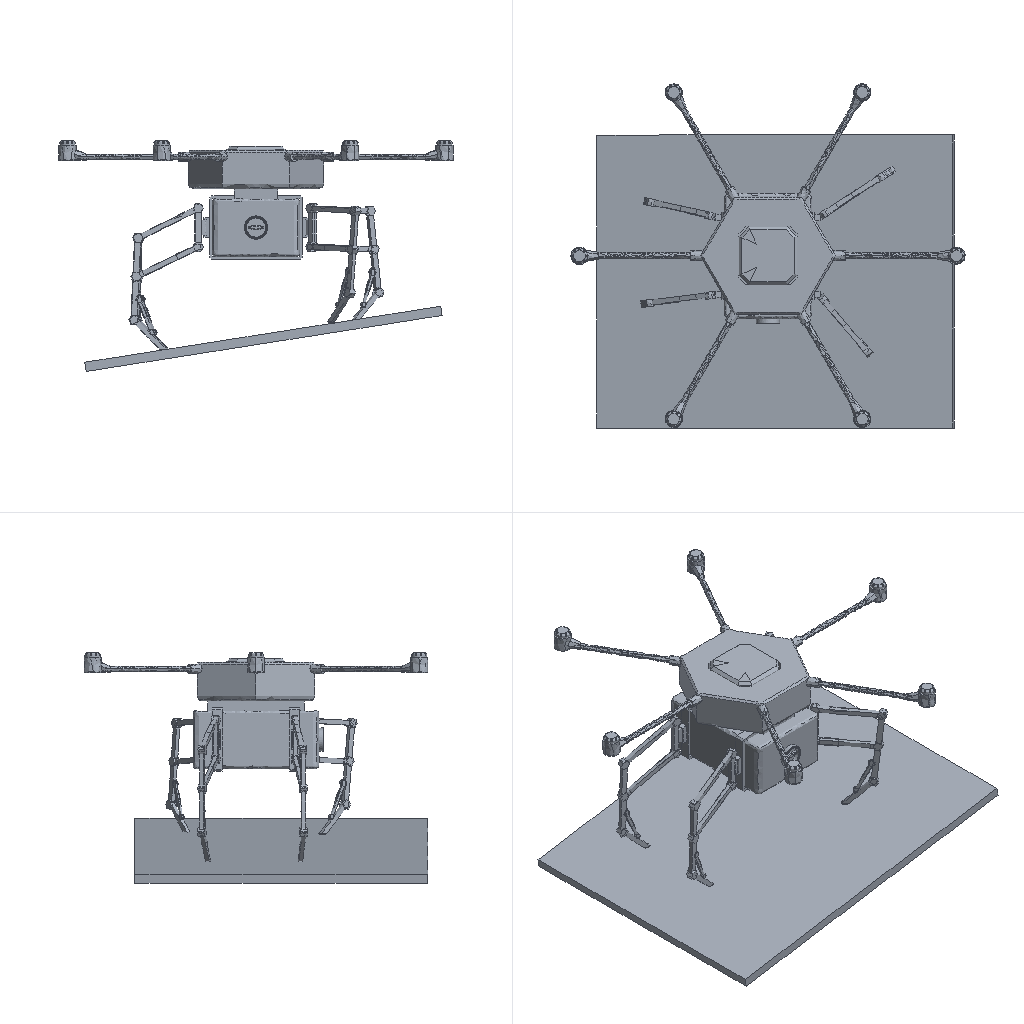Simulation study | ansys workbench
Ansys APDL input file, long lists of numbers shortened:
/batch
/config,noeldb,1     ! force off writing results to database
*get,_wallstrt,active,,time,wall
! ANSYS input file written by Workbench version 2022 R1
! File used for geometry attach:
/title,wbnew--__ (G5)
! ****** Begin Custom Load Command Snippet ******
/COM, ACT Extensions:
/COM,     LSDYNA, 2021.1
/COM,
! ****** End   Custom Load Command Snippet ******
*DIM,_wb_ProjectScratch_dir,string,248
_wb_ProjectScratch_dir(1) = ''
*DIM,_wb_SolverFiles_dir,string,248
_wb_SolverFiles_dir(1) = ''
*DIM,_wb_userfiles_dir,string,248
_wb_userfiles_dir(1) = ''
/com,--- Data in consistent NMM units. See Solving Units in the help system for more information.
/units,MPA
/nopr
/wb,file,start              !  signify a WB generated input file
/prep7
! Turn off shape checking because checks already performed inside WB mesher.
! See help system for more information.
SHPP,OFF,,NOWARN
/nolist
etcon,set             ! allow ANSYS to choose best KEYOP's for 180x elements, resets any applicable keyopt to MAPDL defaults
/com,*********** Nodes for the whole assembly ***********
nblock,3,,112522
(1i9,3e20.9e3)
        1    -5.508865346E+03    -1.475800000E+03    -1.735902488E+03
! (102292 more lines like these left out)
-1
/wb,elem,start            !  set before creation of elements
/com,*********** Elements for Body 1 "xuanyi|dianjizhijia|Chamfer.1" ***********
et,1,187
eblock,19,solid,,480
(19i9)
        1        1        1        1        0        0        0        0       10        0     5151    10218    10222    10326    10253    10413    10440    10416    10414
! (959 more lines like these left out)
-1
/com,*********** Elements for Body 2 "xuanyi|jibi|Pad.1" ***********
et,2,187
eblock,19,solid,,1308
(19i9)
        2        2        2        2        0        0        0        0       10        0    42302    78291    78292    78359    78451    79365    79376    79367    79371
! (2615 more lines like these left out)
-1
/com,*********** Elements for Body 3 "xuanyi|xuanyidianji|CircPattern.1" ***********
et,3,187
eblock,19,solid,,3493
(19i9)
        3        3        3        3        0        0        0        0       10        0     9787    19116    19133    19215    19181    23808    23876    23812    23809
! (6985 more lines like these left out)
-1
/com,*********** Elements for Body 4 "xuanyi|dianjizhijia|Chamfer.1[2]" ***********
et,4,187
eblock,19,solid,,480
(19i9)
        4        4        4        4        0        0        0        0       10        0     4671     9210     9214     9318     9245     9405     9432     9408     9406
! (959 more lines like these left out)
-1
/com,*********** Elements for Body 5 "xuanyi|jibi|Pad.1[2]" ***********
et,5,187
eblock,19,solid,,1308
(19i9)
        5        5        5        5        0        0        0        0       10        0    38378    70386    70387    70454    70546    71460    71471    71462    71466
! (2615 more lines like these left out)
-1
! (50 more sections like these left out)
/wb,elem,end               !  done creating elements
/com,*********** Send User Defined Coordinate System(s) ***********
csys,0
toffst,273.15,  ! Temperature offset from absolute zero
/com,*********** Set Reference Temperature ***********
tref,22.
/wb,mat,start              !  starting to send materials
/com,*********** Send Materials ***********
Temperature = 'TEMP' ! Temperature
MP,DENS,1,7.85e-09,	! tonne mm^-3
MP,ALPX,1,1.2e-05,	! C^-1
MP,C,1,434000000,	! mm^2 s^-2 C^-1
MP,KXX,1,60.5,	! tonne mm s^-3 C^-1
MP,RSVX,1,0.00017,	! ohm mm
MP,EX,1,200000,	! tonne s^-2 mm^-1
MP,NUXY,1,0.3,
MP,MURX,1,10000,
Temperature = 'TEMP' ! Temperature
MP,DENS,2,7.85e-09,	! tonne mm^-3
MP,ALPX,2,1.2e-05,	! C^-1
MP,C,2,434000000,	! mm^2 s^-2 C^-1
MP,KXX,2,60.5,	! tonne mm s^-3 C^-1
MP,RSVX,2,0.00017,	! ohm mm
MP,EX,2,200000,	! tonne s^-2 mm^-1
MP,NUXY,2,0.3,
MP,MURX,2,10000,
Temperature = 'TEMP' ! Temperature
MP,DENS,3,7.85e-09,	! tonne mm^-3
MP,ALPX,3,1.2e-05,	! C^-1
MP,C,3,434000000,	! mm^2 s^-2 C^-1
MP,KXX,3,60.5,	! tonne mm s^-3 C^-1
MP,RSVX,3,0.00017,	! ohm mm
MP,EX,3,200000,	! tonne s^-2 mm^-1
MP,NUXY,3,0.3,
MP,MURX,3,10000,
Temperature = 'TEMP' ! Temperature
MP,DENS,4,7.85e-09,	! tonne mm^-3
MP,ALPX,4,1.2e-05,	! C^-1
MP,C,4,434000000,	! mm^2 s^-2 C^-1
MP,KXX,4,60.5,	! tonne mm s^-3 C^-1
MP,RSVX,4,0.00017,	! ohm mm
MP,EX,4,200000,	! tonne s^-2 mm^-1
MP,NUXY,4,0.3,
MP,MURX,4,10000,
Temperature = 'TEMP' ! Temperature
MP,DENS,5,7.85e-09,	! tonne mm^-3
MP,ALPX,5,1.2e-05,	! C^-1
MP,C,5,434000000,	! mm^2 s^-2 C^-1
MP,KXX,5,60.5,	! tonne mm s^-3 C^-1
MP,RSVX,5,0.00017,	! ohm mm
MP,EX,5,200000,	! tonne s^-2 mm^-1
MP,NUXY,5,0.3,
MP,MURX,5,10000,
Temperature = 'TEMP' ! Temperature
MP,DENS,6,7.85e-09,	! tonne mm^-3
MP,ALPX,6,1.2e-05,	! C^-1
MP,C,6,434000000,	! mm^2 s^-2 C^-1
MP,KXX,6,60.5,	! tonne mm s^-3 C^-1
MP,RSVX,6,0.00017,	! ohm mm
MP,EX,6,200000,	! tonne s^-2 mm^-1
MP,NUXY,6,0.3,
MP,MURX,6,10000,
Temperature = 'TEMP' ! Temperature
MP,DENS,7,7.85e-09,	! tonne mm^-3
MP,ALPX,7,1.2e-05,	! C^-1
MP,C,7,434000000,	! mm^2 s^-2 C^-1
MP,KXX,7,60.5,	! tonne mm s^-3 C^-1
MP,RSVX,7,0.00017,	! ohm mm
MP,EX,7,200000,	! tonne s^-2 mm^-1
MP,NUXY,7,0.3,
MP,MURX,7,10000,
Temperature = 'TEMP' ! Temperature
MP,DENS,8,7.85e-09,	! tonne mm^-3
MP,ALPX,8,1.2e-05,	! C^-1
MP,C,8,434000000,	! mm^2 s^-2 C^-1
MP,KXX,8,60.5,	! tonne mm s^-3 C^-1
MP,RSVX,8,0.00017,	! ohm mm
MP,EX,8,200000,	! tonne s^-2 mm^-1
MP,NUXY,8,0.3,
MP,MURX,8,10000,
Temperature = 'TEMP' ! Temperature
MP,DENS,9,7.85e-09,	! tonne mm^-3
MP,ALPX,9,1.2e-05,	! C^-1
MP,C,9,434000000,	! mm^2 s^-2 C^-1
MP,KXX,9,60.5,	! tonne mm s^-3 C^-1
MP,RSVX,9,0.00017,	! ohm mm
MP,EX,9,200000,	! tonne s^-2 mm^-1
! (416 more lines like these left out)
/wb,mat,end                !  done sending materials
!************************* Model Summary ********************
!xuanyi|dianjizhijia|Chamfer.1,	结构钢,	matid,	1
!xuanyi|jibi|Pad.1,	结构钢,	matid,	2
!xuanyi|xuanyidianji|CircPattern.1,	结构钢,	matid,	3
! (54 more lines like these left out)
*get,_xmin,node,,mnloc,x
*get,_ymin,node,,mnloc,y
*get,_zmin,node,,mnloc,z
*get,_xmax,node,,mxloc,x
*get,_ymax,node,,mxloc,y
*get,_zmax,node,,mxloc,z
_ASMDIAG=(_xmax-_xmin)*(_xmax-_xmin)+(_ymax-_ymin)*(_ymax-_ymin)+(_zmax-_zmin)*(_zmax-_zmin)
_ASMDIAG=SQRT(_ASMDIAG)
/wb,contact,start          !  starting to send contact
/com,*********** Create Contact "接触区域" ***********
/com,            Real Constant Set For Above Contact Is 57 & 56
*set,tid,57
*set,cid,56
r,tid
r,cid
et,tid,170
et,cid,174
eblock,10,,,60
(15i9)
    81076       57       57       57        0    10266    10359    10268    10268    10777    10797    10268    10771
! (59 more lines like these left out)
-1
eblock,10,,,60
(15i9)
    81136       56       56       56        0    10266    10359    10268    10268    10777    10797    10268    10771
! (59 more lines like these left out)
-1
eblock,10,,,74
(15i9)
    81196       56       57       56        0    78221    78228    78223    78223    78711    78720    78223    78709
! (73 more lines like these left out)
-1
eblock,10,,,74
(15i9)
    81270       57       56       57        0    78221    78228    78223    78223    78711    78720    78223    78709
! (73 more lines like these left out)
-1
keyo,cid,8,2               ! auto create asymmetric contact (from Program Controlled setting)
keyo,cid,10,0              ! adjust contact stiffness each NR iteration (from Program Controlled setting)
keyo,cid,12,5              ! bonded always
keyo,cid,18,1              ! small sliding turned on by application
keyo,cid,2,0               ! augmented Lagrange (from Program Controlled setting)
keyo,cid,4,0               ! on Gauss point (from Program Controlled setting)
keyo,cid,9,1               ! ignore initial gaps/penetration
keyo,cid,7,0               ! No Prediction
rmod,tid,3,10.      ! FKN
rmod,tid,5,0.       ! ICONT
rmod,tid,6,0.       ! PINB
rmod,tid,10,0.      ! CNOF
rmod,tid,12,0.      ! FKT
rmod,tid,36,230     ! WB DSID
rmod,cid,3,10.      ! FKN
rmod,cid,5,0.       ! ICONT
rmod,cid,6,0.       ! PINB
rmod,cid,10,0.      ! CNOF
rmod,cid,12,0.      ! FKT
rmod,cid,36,230     ! WB DSID
/com,*********** Create Contact "接触区域 2" ***********
/com,            Real Constant Set For Above Contact Is 59 & 58
*set,tid,59
*set,cid,58
r,tid
r,cid
et,tid,170
et,cid,174
eblock,10,,,78
(15i9)
    81344       59       59       59        0    10248    10250    10360    10360    10635    10655    10360    10640
! (77 more lines like these left out)
-1
eblock,10,,,78
(15i9)
    81422       58       58       58        0    10248    10250    10360    10360    10635    10655    10360    10640
! (77 more lines like these left out)
-1
eblock,10,,,254
(15i9)
    81500       58       59       58        0    18597    18807    18604    18604    20815    20867    18604    20811
! (253 more lines like these left out)
-1
eblock,10,,,254
(15i9)
    81754       59       58       59        0    18597    18807    18604    18604    20815    20867    18604    20811
! (253 more lines like these left out)
-1
keyo,cid,8,2               ! auto create asymmetric contact (from Program Controlled setting)
keyo,cid,10,0              ! adjust contact stiffness each NR iteration (from Program Controlled setting)
keyo,cid,12,5              ! bonded always
keyo,cid,18,1              ! small sliding turned on by application
keyo,cid,2,0               ! augmented Lagrange (from Program Controlled setting)
keyo,cid,4,0               ! on Gauss point (from Program Controlled setting)
keyo,cid,9,1               ! ignore initial gaps/penetration
keyo,cid,7,0               ! No Prediction
rmod,tid,3,10.      ! FKN
rmod,tid,5,0.       ! ICONT
rmod,tid,6,0.       ! PINB
rmod,tid,10,0.      ! CNOF
rmod,tid,12,0.      ! FKT
rmod,tid,36,233     ! WB DSID
rmod,cid,3,10.      ! FKN
rmod,cid,5,0.       ! ICONT
rmod,cid,6,0.       ! PINB
rmod,cid,10,0.      ! CNOF
rmod,cid,12,0.      ! FKT
rmod,cid,36,233     ! WB DSID
/com,*********** Create Contact "接触区域 3" ***********
/com,            Real Constant Set For Above Contact Is 61 & 60
*set,tid,61
*set,cid,60
r,tid
r,cid
et,tid,170
et,cid,174
eblock,10,,,85
(15i9)
    82008       61       61       61        0    78213    78220    78218    78218    78666    78695    78218    78665
! (84 more lines like these left out)
-1
eblock,10,,,85
(15i9)
    82093       60       60       60        0    78213    78220    78218    78218    78666    78695    78218    78665
! (84 more lines like these left out)
-1
eblock,10,,,60
(15i9)
    82178       60       61       60        0    39970    40746    39973    39973    44807    44832    39973    44805
! (59 more lines like these left out)
-1
eblock,10,,,60
(15i9)
    82238       61       60       61        0    39970    40746    39973    39973    44807    44832    39973    44805
! (59 more lines like these left out)
-1
keyo,cid,8,2               ! auto create asymmetric contact (from Program Controlled setting)
keyo,cid,10,0              ! adjust contact stiffness each NR iteration (from Program Controlled setting)
keyo,cid,12,5              ! bonded always
keyo,cid,18,1              ! small sliding turned on by application
keyo,cid,2,0               ! augmented Lagrange (from Program Controlled setting)
keyo,cid,4,0               ! on Gauss point (from Program Controlled setting)
keyo,cid,9,1               ! ignore initial gaps/penetration
keyo,cid,7,0               ! No Prediction
rmod,tid,3,10.      ! FKN
rmod,tid,5,0.       ! ICONT
rmod,tid,6,0.       ! PINB
rmod,tid,10,0.      ! CNOF
rmod,tid,12,0.      ! FKT
rmod,tid,36,236     ! WB DSID
rmod,cid,3,10.      ! FKN
rmod,cid,5,0.       ! ICONT
rmod,cid,6,0.       ! PINB
rmod,cid,10,0.      ! CNOF
rmod,cid,12,0.      ! FKT
rmod,cid,36,236     ! WB DSID
/com,*********** Create Contact "接触区域 8" ***********
/com,            Real Constant Set For Above Contact Is 63 & 62
*set,tid,63
*set,cid,62
r,tid
r,cid
et,tid,170
et,cid,174
eblock,10,,,60
(15i9)
    82298       63       63       63        0     9258     9351     9260     9260     9769     9789     9260     9763
! (59 more lines like these left out)
-1
eblock,10,,,60
(15i9)
    82358       62       62       62        0     9258     9351     9260     9260     9769     9789     9260     9763
! (59 more lines like these left out)
-1
eblock,10,,,74
(15i9)
    82418       62       63       62        0    70316    70323    70318    70318    70806    70815    70318    70804
! (73 more lines like these left out)
-1
eblock,10,,,74
(15i9)
    82492       63       62       63        0    70316    70323    70318    70318    70806    70815    70318    70804
! (73 more lines like these left out)
-1
keyo,cid,8,2               ! auto create asymmetric contact (from Program Controlled setting)
keyo,cid,10,0              ! adjust contact stiffness each NR iteration (from Program Controlled setting)
keyo,cid,12,5              ! bonded always
keyo,cid,18,1              ! small sliding turned on by application
keyo,cid,2,0               ! augmented Lagrange (from Program Controlled setting)
keyo,cid,4,0               ! on Gauss point (from Program Controlled setting)
keyo,cid,9,1               ! ignore initial gaps/penetration
keyo,cid,7,0               ! No Prediction
rmod,tid,3,10.      ! FKN
rmod,tid,5,0.       ! ICONT
rmod,tid,6,0.       ! PINB
rmod,tid,10,0.      ! CNOF
rmod,tid,12,0.      ! FKT
rmod,tid,36,251     ! WB DSID
rmod,cid,3,10.      ! FKN
rmod,cid,5,0.       ! ICONT
rmod,cid,6,0.       ! PINB
rmod,cid,10,0.      ! CNOF
rmod,cid,12,0.      ! FKT
rmod,cid,36,251     ! WB DSID
/com,*********** Create Contact "接触区域 9" ***********
/com,            Real Constant Set For Above Contact Is 65 & 64
*set,tid,65
*set,cid,64
r,tid
r,cid
et,tid,170
et,cid,174
eblock,10,,,78
(15i9)
    82566       65       65       65        0     9240     9242     9352     9352     9627     9647     9352     9632
! (77 more lines like these left out)
-1
eblock,10,,,78
(15i9)
    82644       64       64       64        0     9240     9242     9352     9352     9627     9647     9352     9632
! (77 more lines like these left out)
-1
eblock,10,,,254
(15i9)
    82722       64       65       64        0    12443    12653    12450    12450    14661    14713    12450    14657
! (253 more lines like these left out)
-1
eblock,10,,,254
(15i9)
    82976       65       64       65        0    12443    12653    12450    12450    14661    14713    12450    14657
! (253 more lines like these left out)
-1
keyo,cid,8,2               ! auto create asymmetric contact (from Program Controlled setting)
keyo,cid,10,0              ! adjust contact stiffness each NR iteration (from Program Controlled setting)
keyo,cid,12,5              ! bonded always
keyo,cid,18,1              ! small sliding turned on by application
keyo,cid,2,0               ! augmented Lagrange (from Program Controlled setting)
keyo,cid,4,0               ! on Gauss point (from Program Controlled setting)
keyo,cid,9,1               ! ignore initial gaps/penetration
keyo,cid,7,0               ! No Prediction
rmod,tid,3,10.      ! FKN
rmod,tid,5,0.       ! ICONT
rmod,tid,6,0.       ! PINB
rmod,tid,10,0.      ! CNOF
rmod,tid,12,0.      ! FKT
rmod,tid,36,254     ! WB DSID
rmod,cid,3,10.      ! FKN
rmod,cid,5,0.       ! ICONT
rmod,cid,6,0.       ! PINB
rmod,cid,10,0.      ! CNOF
rmod,cid,12,0.      ! FKT
rmod,cid,36,254     ! WB DSID
! (62 more sections like these left out)
/wb,contact,end            !  done creating contacts
/golist
/wb,load,start             !  starting to send loads
/com,*********** Fixed Supports ***********
CMBLOCK,_FIXEDSU,NODE,     6538
(8i10)
         1         2         3         4         5         6         7         8
! (817 more lines like these left out)
cmsel,s,_FIXEDSU
d,all,all
nsel,all
/com,*********** Define Force Using Surface Effect Elements ***********
local,12,0,0.,0.,0.,0.,0.,0.
csys,0
et,190,154
eblock,10,,,642
(15i9)
    93924      190      190      190       12    40598    40641    40621    40621    48073    48267    40621    48071
! (641 more lines like these left out)
-1
esel,s,type,,190
keyop,190,2,1                ! Apply load in local coordinate system
keyop,190,7,1                ! Use original area so load is constant in large deformation
esel,all
/gst,on,on
fini
*get,_numnode,node,0,count
*get,_numelem,elem,0,count
*get, _MAXELEMNUM, elem, 0, NUM, MAX
*get, _MAXNODENUM, node, 0, NUM, MAX
*get, _MAXELEMTYPE, etyp, 0, NUM, MAX
*get, _MAXREALCONST, real, 0, NUM, MAX
/go
/wb,load,end               !  done creating loads
/com,--- Number of total nodes = %_numnode%
/com,--- Number of contact elements = 13490
/com,--- Number of spring elements = 0
/com,--- Number of bearing elements = 0
/com,--- Number of solid elements = 55575
/com,--- Number of condensed parts = 0
/com,--- Number of total elements = %_numelem%
*get,_wallbsol,active,,time,wall
/com,****************************************************************************
/com,*************************    SOLUTION       ********************************
/com,****************************************************************************
/solu
antype,4                   ! transient analysis
nlgeom,on                  ! Turn on Large Deformation Effects
kbc,1                      ! stepped BC's
_thickRatio=0.164   ! Ratio of thick parts in the model
eqsl,sparse,,,,,1
cntr,print,1               ! print out contact info and also make no initial contact an error
dmpoption,emat,no             ! Don't combine emat file for DANSYS
dmpoption,esav,no             ! Don't combine esav file for DANSYS
trnopt,full,,,,,hht        ! HHT time integration method
tintp, mosp			! Choose transient integration settings for moderate speed application
nldiag,cont,iter           ! print out contact info each equilibrium iteration
rescontrol,define,last,last,,dele	   ! Program Controlled
/com,****************************************************
/com,******************* SOLVE FOR LS 1 OF 1 ****************
esel,s,type,,190
nsle
sfe,all,1,pres,1,0.
sfe,all,2,pres,1,0.
sfe,all,3,pres,1,-2.328
nsel,all
esel,all
acel,0.,0.,-84.28
/nopr
/gopr
autots,on                   ! User turned on automatic time stepping
deltim,1,1,1,OFF
time,1.
timint,on                  ! Turn on time integration effects
outres,erase
outres,all,none
outres,nsol,all,
outres,rsol,all
outres,eangl,all
outres,etmp,all
outres,veng,all
outres,strs,all,
outres,epel,all,
outres,eppl,all,
outres,cont,all,
outres,v,all,
outres,a,all,
! *********** WB SOLVE COMMAND ***********
! check interactive state
*get,ANSINTER_,active,,int
*if,ANSINTER_,ne,0,then
/eof
*endif
solve
/com *************** Write FE CONNECTORS *********
CEWRITE,file,ce,,INTE
/com,****************************************************
/com,*************** FINISHED SOLVE FOR LS 1 *************
*get,_wallasol,active,,time,wall
/nopr
*get,_numnode,node,0,count
*get,_numelem,elem,0,count
*get, _MAXELEMNUM, elem, 0, NUM, MAX
*get, _MAXNODENUM, node, 0, NUM, MAX,,,INTERNAL
*get, _MAXELEMTYPE, etyp, 0, NUM, MAX
*get, _MAXREALCONST, real, 0, NUM, MAX
/gopr
/post1
xmlo,ENCODING,ISO-8859-1
xmlo,parm
/xml,parm,xml
fini
/gopr
*get,_walldone,active,,time,wall
_preptime=(_wallbsol-_wallstrt)*3600
_solvtime=(_wallasol-_wallbsol)*3600
_posttime=(_walldone-_wallasol)*3600
_totaltim=(_walldone-_wallstrt)*3600
*get,_dlbratio,active,0,solu,dlbr
*get,_combtime,active,0,solu,comb
*get,_ssmode,active,0,solu,ssmm
*get,_ndofs,active,0,solu,ndof
*get,_sol_end_time,active,0,set,time
*if,_sol_end_time,eq,1.,then
/fclean				!clean distributed files
*endif
/com,--- Total number of nodes = %_numnode%
/com,--- Total number of elements = %_numelem%
/com,--- Element load balance ratio = %_dlbratio%
/com,--- Time to combine distributed files = %_combtime%
/com,--- Sparse memory mode = %_ssmode%
/com,--- Number of DOF = %_ndofs%
/wb,file,end               ! done with WB generated input